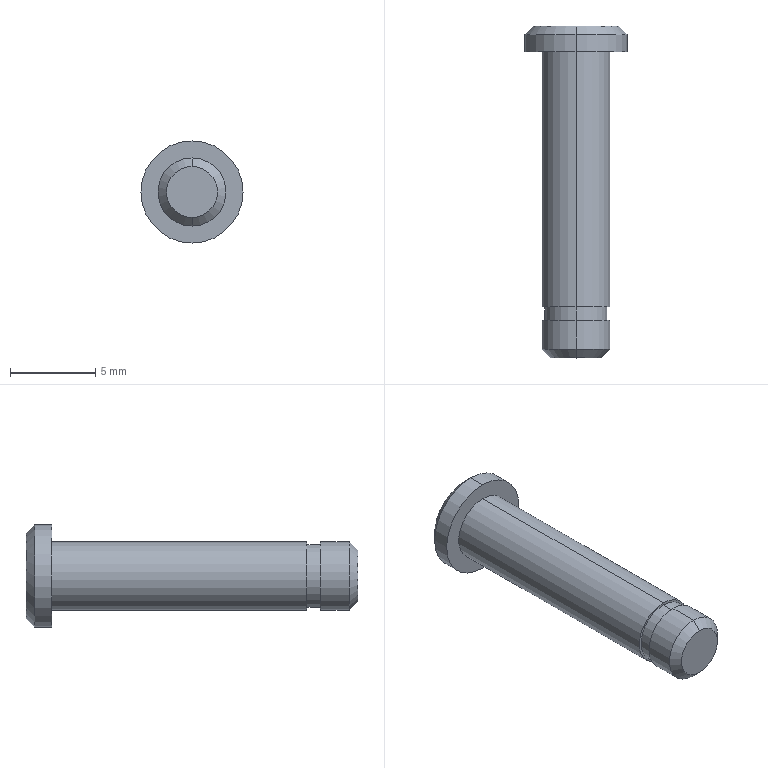Part | SolidWorks | features Chamfer 2, Extrusion 1, ICE 1, RevCut 1 | 1 solid | 17 faces | box 6 x 19.5 x 6 mm | volume 263.49 mm3 | cylinder 8 | plane 5 | cone 4 | commonest cylinder face diameters 4 x4 3.7 x2 6 x2
STEP:
#1=CARTESIAN_POINT('',(0.,-18.,-1.5));
#2=VERTEX_POINT('',#1);
#3=CARTESIAN_POINT('',(0.,-18.,1.5));
#4=VERTEX_POINT('',#3);
#5=CARTESIAN_POINT('',(0.,-18.,0.));
#6=DIRECTION('',(0.,-1.,0.));
#7=DIRECTION('',(0.,0.,-1.));
#8=AXIS2_PLACEMENT_3D('',#5,#6,#7);
#9=CIRCLE('',#8,1.5);
#10=EDGE_CURVE('',#2,#4,#9,.T.);
#11=ORIENTED_EDGE('',*,*,#10,.F.);
#12=CARTESIAN_POINT('',(0.,-17.5,-2.));
#13=VERTEX_POINT('',#12);
#14=CARTESIAN_POINT('',(0.,-18.,-1.5));
#15=DIRECTION('',(0.,0.7071,-0.7071));
#16=VECTOR('',#15,1000.);
#17=LINE('',#14,#16);
#18=EDGE_CURVE('',#2,#13,#17,.T.);
#19=ORIENTED_EDGE('',*,*,#18,.T.);
#20=CARTESIAN_POINT('',(0.,-17.5,2.));
#21=VERTEX_POINT('',#20);
#22=CARTESIAN_POINT('',(0.,-17.5,0.));
#23=DIRECTION('',(0.,1.,0.));
#24=DIRECTION('',(0.,0.,-1.));
#25=AXIS2_PLACEMENT_3D('',#22,#23,#24);
#26=CIRCLE('',#25,2.);
#27=EDGE_CURVE('',#21,#13,#26,.T.);
#28=ORIENTED_EDGE('',*,*,#27,.F.);
#29=CARTESIAN_POINT('',(0.,-18.,1.5));
#30=DIRECTION('',(0.,0.7071,0.7071));
#31=VECTOR('',#30,1000.);
#32=LINE('',#29,#31);
#33=EDGE_CURVE('',#4,#21,#32,.T.);
#34=ORIENTED_EDGE('',*,*,#33,.F.);
#35=EDGE_LOOP('',(#11,#19,#28,#34));
#36=FACE_OUTER_BOUND('',#35,.T.);
#37=CARTESIAN_POINT('',(0.,-18.,0.));
#38=DIRECTION('',(0.,1.,0.));
#39=DIRECTION('',(0.,0.,1.));
#40=AXIS2_PLACEMENT_3D('',#37,#38,#39);
#41=CONICAL_SURFACE('',#40,1.5,0.7854);
#42=ADVANCED_FACE('',(#36),#41,.T.);
#43=CARTESIAN_POINT('',(0.,1.5,2.5));
#44=VERTEX_POINT('',#43);
#45=CARTESIAN_POINT('',(0.,1.5,-2.5));
#46=VERTEX_POINT('',#45);
#47=CARTESIAN_POINT('',(0.,1.5,0.));
#48=DIRECTION('',(0.,1.,0.));
#49=DIRECTION('',(0.,0.,1.));
#50=AXIS2_PLACEMENT_3D('',#47,#48,#49);
#51=CIRCLE('',#50,2.5);
#52=EDGE_CURVE('',#44,#46,#51,.T.);
#53=ORIENTED_EDGE('',*,*,#52,.F.);
#54=CARTESIAN_POINT('',(0.,1.,3.));
#55=VERTEX_POINT('',#54);
#56=CARTESIAN_POINT('',(0.,1.5,2.5));
#57=DIRECTION('',(0.,-0.7071,0.7071));
#58=VECTOR('',#57,1000.);
#59=LINE('',#56,#58);
#60=EDGE_CURVE('',#44,#55,#59,.T.);
#61=ORIENTED_EDGE('',*,*,#60,.T.);
#62=CARTESIAN_POINT('',(0.,1.,-3.));
#63=VERTEX_POINT('',#62);
#64=CARTESIAN_POINT('',(0.,1.,0.));
#65=DIRECTION('',(0.,-1.,0.));
#66=DIRECTION('',(0.,0.,1.));
#67=AXIS2_PLACEMENT_3D('',#64,#65,#66);
#68=CIRCLE('',#67,3.);
#69=EDGE_CURVE('',#63,#55,#68,.T.);
#70=ORIENTED_EDGE('',*,*,#69,.F.);
#71=CARTESIAN_POINT('',(0.,1.5,-2.5));
#72=DIRECTION('',(0.,-0.7071,-0.7071));
#73=VECTOR('',#72,1000.);
#74=LINE('',#71,#73);
#75=EDGE_CURVE('',#46,#63,#74,.T.);
#76=ORIENTED_EDGE('',*,*,#75,.F.);
#77=EDGE_LOOP('',(#53,#61,#70,#76));
#78=FACE_OUTER_BOUND('',#77,.T.);
#79=CARTESIAN_POINT('',(0.,1.5,0.));
#80=DIRECTION('',(0.,-1.,0.));
#81=DIRECTION('',(0.,0.,-1.));
#82=AXIS2_PLACEMENT_3D('',#79,#80,#81);
#83=CONICAL_SURFACE('',#82,2.5,0.7854);
#84=ADVANCED_FACE('',(#78),#83,.T.);
#85=ORIENTED_EDGE('',*,*,#27,.T.);
#86=CARTESIAN_POINT('',(0.,-15.8,-2.));
#87=VERTEX_POINT('',#86);
#88=CARTESIAN_POINT('',(0.,-18.,-2.));
#89=DIRECTION('',(0.,1.,0.));
#90=VECTOR('',#89,1000.);
#91=LINE('',#88,#90);
#92=EDGE_CURVE('',#13,#87,#91,.T.);
#93=ORIENTED_EDGE('',*,*,#92,.T.);
#94=CARTESIAN_POINT('',(0.,-15.8,2.));
#95=VERTEX_POINT('',#94);
#96=CARTESIAN_POINT('',(0.,-15.8,0.));
#97=DIRECTION('',(0.,-1.,0.));
#98=DIRECTION('',(0.,0.,-1.));
#99=AXIS2_PLACEMENT_3D('',#96,#97,#98);
#100=CIRCLE('',#99,2.);
#101=EDGE_CURVE('',#87,#95,#100,.T.);
#102=ORIENTED_EDGE('',*,*,#101,.T.);
#103=CARTESIAN_POINT('',(0.,-18.,2.));
#104=DIRECTION('',(0.,1.,0.));
#105=VECTOR('',#104,1000.);
#106=LINE('',#103,#105);
#107=EDGE_CURVE('',#21,#95,#106,.T.);
#108=ORIENTED_EDGE('',*,*,#107,.F.);
#109=EDGE_LOOP('',(#85,#93,#102,#108));
#110=FACE_OUTER_BOUND('',#109,.T.);
#111=CARTESIAN_POINT('',(0.,-18.,0.));
#112=DIRECTION('',(0.,1.,0.));
#113=DIRECTION('',(0.,0.,1.));
#114=AXIS2_PLACEMENT_3D('',#111,#112,#113);
#115=CYLINDRICAL_SURFACE('',#114,2.);
#116=ADVANCED_FACE('',(#110),#115,.T.);
#117=CARTESIAN_POINT('',(0.,-15.,-1.85));
#118=VERTEX_POINT('',#117);
#119=CARTESIAN_POINT('',(0.,-15.,1.85));
#120=VERTEX_POINT('',#119);
#121=CARTESIAN_POINT('',(0.,-15.,0.));
#122=DIRECTION('',(0.,-1.,0.));
#123=DIRECTION('',(0.,0.,-1.));
#124=AXIS2_PLACEMENT_3D('',#121,#122,#123);
#125=CIRCLE('',#124,1.85);
#126=EDGE_CURVE('',#118,#120,#125,.T.);
#127=ORIENTED_EDGE('',*,*,#126,.T.);
#128=CARTESIAN_POINT('',(0.,-15.8,1.85));
#129=VERTEX_POINT('',#128);
#130=CARTESIAN_POINT('',(0.,-16.563,1.85));
#131=DIRECTION('',(0.,-1.,0.));
#132=VECTOR('',#131,1000.);
#133=LINE('',#130,#132);
#134=EDGE_CURVE('',#120,#129,#133,.T.);
#135=ORIENTED_EDGE('',*,*,#134,.T.);
#136=CARTESIAN_POINT('',(0.,-15.8,-1.85));
#137=VERTEX_POINT('',#136);
#138=CARTESIAN_POINT('',(0.,-15.8,0.));
#139=DIRECTION('',(0.,-1.,0.));
#140=DIRECTION('',(0.,0.,-1.));
#141=AXIS2_PLACEMENT_3D('',#138,#139,#140);
#142=CIRCLE('',#141,1.85);
#143=EDGE_CURVE('',#137,#129,#142,.T.);
#144=ORIENTED_EDGE('',*,*,#143,.F.);
#145=CARTESIAN_POINT('',(0.,-16.563,-1.85));
#146=DIRECTION('',(0.,-1.,0.));
#147=VECTOR('',#146,1000.);
#148=LINE('',#145,#147);
#149=EDGE_CURVE('',#118,#137,#148,.T.);
#150=ORIENTED_EDGE('',*,*,#149,.F.);
#151=EDGE_LOOP('',(#127,#135,#144,#150));
#152=FACE_OUTER_BOUND('',#151,.T.);
#153=CARTESIAN_POINT('',(0.,-16.563,0.));
#154=DIRECTION('',(0.,-1.,0.));
#155=DIRECTION('',(0.,0.,-1.));
#156=AXIS2_PLACEMENT_3D('',#153,#154,#155);
#157=CYLINDRICAL_SURFACE('',#156,1.85);
#158=ADVANCED_FACE('',(#152),#157,.T.);
#159=CARTESIAN_POINT('',(0.,-15.,-2.));
#160=VERTEX_POINT('',#159);
#161=CARTESIAN_POINT('',(0.,-15.,2.));
#162=VERTEX_POINT('',#161);
#163=CARTESIAN_POINT('',(0.,-15.,0.));
#164=DIRECTION('',(0.,-1.,0.));
#165=DIRECTION('',(0.,0.,-1.));
#166=AXIS2_PLACEMENT_3D('',#163,#164,#165);
#167=CIRCLE('',#166,2.);
#168=EDGE_CURVE('',#160,#162,#167,.T.);
#169=ORIENTED_EDGE('',*,*,#168,.F.);
#170=CARTESIAN_POINT('',(0.,0.,-2.));
#171=VERTEX_POINT('',#170);
#172=CARTESIAN_POINT('',(0.,-18.,-2.));
#173=DIRECTION('',(0.,1.,0.));
#174=VECTOR('',#173,1000.);
#175=LINE('',#172,#174);
#176=EDGE_CURVE('',#160,#171,#175,.T.);
#177=ORIENTED_EDGE('',*,*,#176,.T.);
#178=CARTESIAN_POINT('',(0.,0.,2.));
#179=VERTEX_POINT('',#178);
#180=CARTESIAN_POINT('',(0.,0.,0.));
#181=DIRECTION('',(0.,-1.,0.));
#182=DIRECTION('',(0.,0.,1.));
#183=AXIS2_PLACEMENT_3D('',#180,#181,#182);
#184=CIRCLE('',#183,2.);
#185=EDGE_CURVE('',#171,#179,#184,.T.);
#186=ORIENTED_EDGE('',*,*,#185,.T.);
#187=CARTESIAN_POINT('',(0.,-18.,2.));
#188=DIRECTION('',(0.,1.,0.));
#189=VECTOR('',#188,1000.);
#190=LINE('',#187,#189);
#191=EDGE_CURVE('',#162,#179,#190,.T.);
#192=ORIENTED_EDGE('',*,*,#191,.F.);
#193=EDGE_LOOP('',(#169,#177,#186,#192));
#194=FACE_OUTER_BOUND('',#193,.T.);
#195=CARTESIAN_POINT('',(0.,-18.,0.));
#196=DIRECTION('',(0.,1.,0.));
#197=DIRECTION('',(0.,0.,1.));
#198=AXIS2_PLACEMENT_3D('',#195,#196,#197);
#199=CYLINDRICAL_SURFACE('',#198,2.);
#200=ADVANCED_FACE('',(#194),#199,.T.);
#201=ORIENTED_EDGE('',*,*,#69,.T.);
#202=CARTESIAN_POINT('',(0.,0.,3.));
#203=VERTEX_POINT('',#202);
#204=CARTESIAN_POINT('',(0.,1.5,3.));
#205=DIRECTION('',(0.,-1.,0.));
#206=VECTOR('',#205,1000.);
#207=LINE('',#204,#206);
#208=EDGE_CURVE('',#55,#203,#207,.T.);
#209=ORIENTED_EDGE('',*,*,#208,.T.);
#210=CARTESIAN_POINT('',(0.,0.,-3.));
#211=VERTEX_POINT('',#210);
#212=CARTESIAN_POINT('',(0.,0.,0.));
#213=DIRECTION('',(0.,1.,0.));
#214=DIRECTION('',(0.,0.,1.));
#215=AXIS2_PLACEMENT_3D('',#212,#213,#214);
#216=CIRCLE('',#215,3.);
#217=EDGE_CURVE('',#203,#211,#216,.T.);
#218=ORIENTED_EDGE('',*,*,#217,.T.);
#219=CARTESIAN_POINT('',(0.,1.5,-3.));
#220=DIRECTION('',(0.,-1.,0.));
#221=VECTOR('',#220,1000.);
#222=LINE('',#219,#221);
#223=EDGE_CURVE('',#63,#211,#222,.T.);
#224=ORIENTED_EDGE('',*,*,#223,.F.);
#225=EDGE_LOOP('',(#201,#209,#218,#224));
#226=FACE_OUTER_BOUND('',#225,.T.);
#227=CARTESIAN_POINT('',(0.,1.5,0.));
#228=DIRECTION('',(0.,-1.,0.));
#229=DIRECTION('',(0.,0.,-1.));
#230=AXIS2_PLACEMENT_3D('',#227,#228,#229);
#231=CYLINDRICAL_SURFACE('',#230,3.);
#232=ADVANCED_FACE('',(#226),#231,.T.);
#233=CARTESIAN_POINT('',(0.,0.,0.));
#234=DIRECTION('',(0.,1.,0.));
#235=DIRECTION('',(0.,0.,1.));
#236=AXIS2_PLACEMENT_3D('',#233,#234,#235);
#237=CIRCLE('',#236,3.);
#238=EDGE_CURVE('',#211,#203,#237,.T.);
#239=ORIENTED_EDGE('',*,*,#238,.F.);
#240=ORIENTED_EDGE('',*,*,#217,.F.);
#241=EDGE_LOOP('',(#239,#240));
#242=FACE_OUTER_BOUND('',#241,.T.);
#243=CARTESIAN_POINT('',(0.,0.,0.));
#244=DIRECTION('',(0.,-1.,0.));
#245=DIRECTION('',(0.,0.,1.));
#246=AXIS2_PLACEMENT_3D('',#243,#244,#245);
#247=CIRCLE('',#246,2.);
#248=EDGE_CURVE('',#179,#171,#247,.T.);
#249=ORIENTED_EDGE('',*,*,#248,.F.);
#250=ORIENTED_EDGE('',*,*,#185,.F.);
#251=EDGE_LOOP('',(#249,#250));
#252=FACE_BOUND('',#251,.T.);
#253=CARTESIAN_POINT('',(0.,0.,0.));
#254=DIRECTION('',(0.,1.,0.));
#255=DIRECTION('',(0.,0.,1.));
#256=AXIS2_PLACEMENT_3D('',#253,#254,#255);
#257=PLANE('',#256);
#258=ADVANCED_FACE('',(#242,#252),#257,.F.);
#259=ORIENTED_EDGE('',*,*,#208,.F.);
#260=CARTESIAN_POINT('',(0.,1.,0.));
#261=DIRECTION('',(0.,-1.,0.));
#262=DIRECTION('',(0.,0.,1.));
#263=AXIS2_PLACEMENT_3D('',#260,#261,#262);
#264=CIRCLE('',#263,3.);
#265=EDGE_CURVE('',#55,#63,#264,.T.);
#266=ORIENTED_EDGE('',*,*,#265,.T.);
#267=ORIENTED_EDGE('',*,*,#223,.T.);
#268=ORIENTED_EDGE('',*,*,#238,.T.);
#269=EDGE_LOOP('',(#259,#266,#267,#268));
#270=FACE_OUTER_BOUND('',#269,.T.);
#271=CARTESIAN_POINT('',(0.,1.5,0.));
#272=DIRECTION('',(0.,-1.,0.));
#273=DIRECTION('',(0.,0.,-1.));
#274=AXIS2_PLACEMENT_3D('',#271,#272,#273);
#275=CYLINDRICAL_SURFACE('',#274,3.);
#276=ADVANCED_FACE('',(#270),#275,.T.);
#277=CARTESIAN_POINT('',(0.,1.5,0.));
#278=DIRECTION('',(0.,1.,0.));
#279=DIRECTION('',(0.,0.,1.));
#280=AXIS2_PLACEMENT_3D('',#277,#278,#279);
#281=CIRCLE('',#280,2.5);
#282=EDGE_CURVE('',#46,#44,#281,.T.);
#283=ORIENTED_EDGE('',*,*,#282,.T.);
#284=ORIENTED_EDGE('',*,*,#52,.T.);
#285=EDGE_LOOP('',(#283,#284));
#286=FACE_OUTER_BOUND('',#285,.T.);
#287=CARTESIAN_POINT('',(0.,1.5,0.));
#288=DIRECTION('',(0.,1.,0.));
#289=DIRECTION('',(0.,0.,1.));
#290=AXIS2_PLACEMENT_3D('',#287,#288,#289);
#291=PLANE('',#290);
#292=ADVANCED_FACE('',(#286),#291,.T.);
#293=ORIENTED_EDGE('',*,*,#176,.F.);
#294=CARTESIAN_POINT('',(0.,-15.,0.));
#295=DIRECTION('',(0.,-1.,0.));
#296=DIRECTION('',(0.,0.,-1.));
#297=AXIS2_PLACEMENT_3D('',#294,#295,#296);
#298=CIRCLE('',#297,2.);
#299=EDGE_CURVE('',#162,#160,#298,.T.);
#300=ORIENTED_EDGE('',*,*,#299,.F.);
#301=ORIENTED_EDGE('',*,*,#191,.T.);
#302=ORIENTED_EDGE('',*,*,#248,.T.);
#303=EDGE_LOOP('',(#293,#300,#301,#302));
#304=FACE_OUTER_BOUND('',#303,.T.);
#305=CARTESIAN_POINT('',(0.,-18.,0.));
#306=DIRECTION('',(0.,1.,0.));
#307=DIRECTION('',(0.,0.,1.));
#308=AXIS2_PLACEMENT_3D('',#305,#306,#307);
#309=CYLINDRICAL_SURFACE('',#308,2.);
#310=ADVANCED_FACE('',(#304),#309,.T.);
#311=CARTESIAN_POINT('',(0.,-15.8,0.));
#312=DIRECTION('',(0.,-1.,0.));
#313=DIRECTION('',(0.,0.,-1.));
#314=AXIS2_PLACEMENT_3D('',#311,#312,#313);
#315=CIRCLE('',#314,2.);
#316=EDGE_CURVE('',#95,#87,#315,.T.);
#317=ORIENTED_EDGE('',*,*,#316,.F.);
#318=ORIENTED_EDGE('',*,*,#101,.F.);
#319=EDGE_LOOP('',(#317,#318));
#320=FACE_OUTER_BOUND('',#319,.T.);
#321=ORIENTED_EDGE('',*,*,#143,.T.);
#322=CARTESIAN_POINT('',(0.,-15.8,0.));
#323=DIRECTION('',(0.,-1.,0.));
#324=DIRECTION('',(0.,0.,-1.));
#325=AXIS2_PLACEMENT_3D('',#322,#323,#324);
#326=CIRCLE('',#325,1.85);
#327=EDGE_CURVE('',#129,#137,#326,.T.);
#328=ORIENTED_EDGE('',*,*,#327,.T.);
#329=EDGE_LOOP('',(#321,#328));
#330=FACE_BOUND('',#329,.T.);
#331=CARTESIAN_POINT('',(0.,-15.8,-2.));
#332=DIRECTION('',(0.,-1.,0.));
#333=DIRECTION('',(0.,0.,-1.));
#334=AXIS2_PLACEMENT_3D('',#331,#332,#333);
#335=PLANE('',#334);
#336=ADVANCED_FACE('',(#320,#330),#335,.F.);
#337=ORIENTED_EDGE('',*,*,#134,.F.);
#338=CARTESIAN_POINT('',(0.,-15.,0.));
#339=DIRECTION('',(0.,-1.,0.));
#340=DIRECTION('',(0.,0.,-1.));
#341=AXIS2_PLACEMENT_3D('',#338,#339,#340);
#342=CIRCLE('',#341,1.85);
#343=EDGE_CURVE('',#120,#118,#342,.T.);
#344=ORIENTED_EDGE('',*,*,#343,.T.);
#345=ORIENTED_EDGE('',*,*,#149,.T.);
#346=ORIENTED_EDGE('',*,*,#327,.F.);
#347=EDGE_LOOP('',(#337,#344,#345,#346));
#348=FACE_OUTER_BOUND('',#347,.T.);
#349=CARTESIAN_POINT('',(0.,-16.563,0.));
#350=DIRECTION('',(0.,-1.,0.));
#351=DIRECTION('',(0.,0.,-1.));
#352=AXIS2_PLACEMENT_3D('',#349,#350,#351);
#353=CYLINDRICAL_SURFACE('',#352,1.85);
#354=ADVANCED_FACE('',(#348),#353,.T.);
#355=ORIENTED_EDGE('',*,*,#126,.F.);
#356=ORIENTED_EDGE('',*,*,#343,.F.);
#357=EDGE_LOOP('',(#355,#356));
#358=FACE_BOUND('',#357,.T.);
#359=ORIENTED_EDGE('',*,*,#299,.T.);
#360=ORIENTED_EDGE('',*,*,#168,.T.);
#361=EDGE_LOOP('',(#359,#360));
#362=FACE_OUTER_BOUND('',#361,.T.);
#363=CARTESIAN_POINT('',(0.,-15.,-2.));
#364=DIRECTION('',(0.,1.,0.));
#365=DIRECTION('',(0.,0.,1.));
#366=AXIS2_PLACEMENT_3D('',#363,#364,#365);
#367=PLANE('',#366);
#368=ADVANCED_FACE('',(#358,#362),#367,.F.);
#369=CARTESIAN_POINT('',(0.,-18.,0.));
#370=DIRECTION('',(0.,-1.,0.));
#371=DIRECTION('',(0.,0.,-1.));
#372=AXIS2_PLACEMENT_3D('',#369,#370,#371);
#373=CIRCLE('',#372,1.5);
#374=EDGE_CURVE('',#4,#2,#373,.T.);
#375=ORIENTED_EDGE('',*,*,#374,.T.);
#376=ORIENTED_EDGE('',*,*,#10,.T.);
#377=EDGE_LOOP('',(#375,#376));
#378=FACE_OUTER_BOUND('',#377,.T.);
#379=CARTESIAN_POINT('',(0.,-18.,0.));
#380=DIRECTION('',(0.,-1.,0.));
#381=DIRECTION('',(0.,0.,-1.));
#382=AXIS2_PLACEMENT_3D('',#379,#380,#381);
#383=PLANE('',#382);
#384=ADVANCED_FACE('',(#378),#383,.T.);
#385=ORIENTED_EDGE('',*,*,#92,.F.);
#386=CARTESIAN_POINT('',(0.,-17.5,0.));
#387=DIRECTION('',(0.,1.,0.));
#388=DIRECTION('',(0.,0.,-1.));
#389=AXIS2_PLACEMENT_3D('',#386,#387,#388);
#390=CIRCLE('',#389,2.);
#391=EDGE_CURVE('',#13,#21,#390,.T.);
#392=ORIENTED_EDGE('',*,*,#391,.T.);
#393=ORIENTED_EDGE('',*,*,#107,.T.);
#394=ORIENTED_EDGE('',*,*,#316,.T.);
#395=EDGE_LOOP('',(#385,#392,#393,#394));
#396=FACE_OUTER_BOUND('',#395,.T.);
#397=CARTESIAN_POINT('',(0.,-18.,0.));
#398=DIRECTION('',(0.,1.,0.));
#399=DIRECTION('',(0.,0.,1.));
#400=AXIS2_PLACEMENT_3D('',#397,#398,#399);
#401=CYLINDRICAL_SURFACE('',#400,2.);
#402=ADVANCED_FACE('',(#396),#401,.T.);
#403=ORIENTED_EDGE('',*,*,#60,.F.);
#404=ORIENTED_EDGE('',*,*,#282,.F.);
#405=ORIENTED_EDGE('',*,*,#75,.T.);
#406=ORIENTED_EDGE('',*,*,#265,.F.);
#407=EDGE_LOOP('',(#403,#404,#405,#406));
#408=FACE_OUTER_BOUND('',#407,.T.);
#409=CARTESIAN_POINT('',(0.,1.5,0.));
#410=DIRECTION('',(0.,-1.,0.));
#411=DIRECTION('',(0.,0.,-1.));
#412=AXIS2_PLACEMENT_3D('',#409,#410,#411);
#413=CONICAL_SURFACE('',#412,2.5,0.7854);
#414=ADVANCED_FACE('',(#408),#413,.T.);
#415=ORIENTED_EDGE('',*,*,#18,.F.);
#416=ORIENTED_EDGE('',*,*,#374,.F.);
#417=ORIENTED_EDGE('',*,*,#33,.T.);
#418=ORIENTED_EDGE('',*,*,#391,.F.);
#419=EDGE_LOOP('',(#415,#416,#417,#418));
#420=FACE_OUTER_BOUND('',#419,.T.);
#421=CARTESIAN_POINT('',(0.,-18.,0.));
#422=DIRECTION('',(0.,1.,0.));
#423=DIRECTION('',(0.,0.,1.));
#424=AXIS2_PLACEMENT_3D('',#421,#422,#423);
#425=CONICAL_SURFACE('',#424,1.5,0.7854);
#426=ADVANCED_FACE('',(#420),#425,.T.);
#427=CLOSED_SHELL('',(#42,#84,#116,#158,#200,#232,#258,#276,#292,#310,#336,#354,#368,#384,#402,#414,#426));
#428=MANIFOLD_SOLID_BREP('',#427);
#429=CARTESIAN_POINT('',(0.,0.,0.));
#430=DIRECTION('',(0.,0.,1.));
#431=DIRECTION('',(1.,0.,0.));
#432=AXIS2_PLACEMENT_3D('',#429,#430,#431);
#433=(LENGTH_UNIT()NAMED_UNIT(*)SI_UNIT(.MILLI.,.METRE.));
#434=UNCERTAINTY_MEASURE_WITH_UNIT(LENGTH_MEASURE(0.00001),#433,'','');
#435=(NAMED_UNIT(*)PLANE_ANGLE_UNIT()SI_UNIT($,.RADIAN.));
#436=(NAMED_UNIT(*)SI_UNIT($,.STERADIAN.)SOLID_ANGLE_UNIT());
#437=(GEOMETRIC_REPRESENTATION_CONTEXT(3)GLOBAL_UNCERTAINTY_ASSIGNED_CONTEXT((#434))GLOBAL_UNIT_ASSIGNED_CONTEXT((#433,#435,#436))REPRESENTATION_CONTEXT('',''));
#438=ADVANCED_BREP_SHAPE_REPRESENTATION('',(#428,#432),#437);